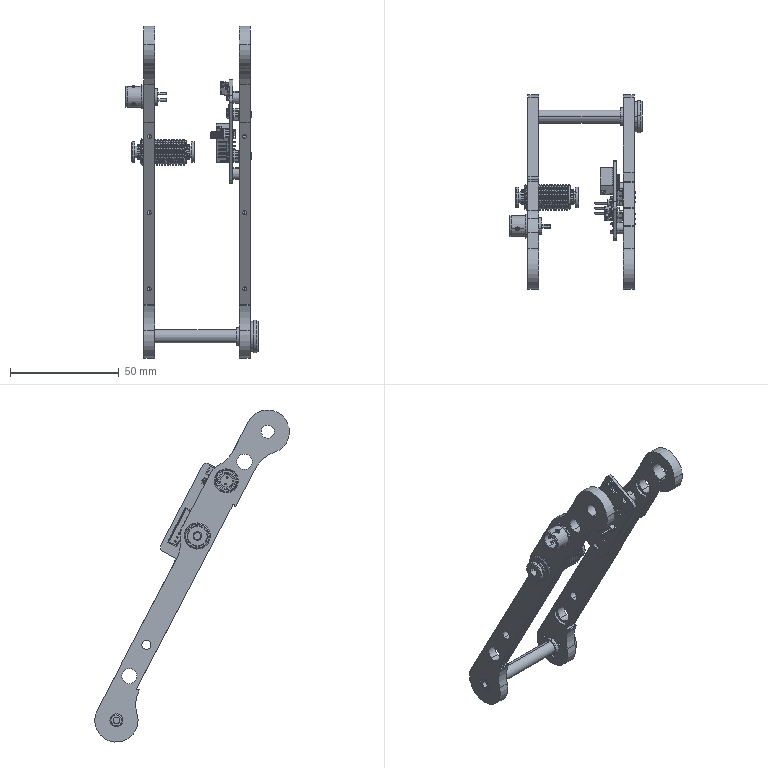Part | NX | features BREP 185 | 185 solids | 2496 faces | box 60.8 x 89.643 x 152.852 mm | volume 26403 mm3 | plane 1478 | cylinder 507 | spline 453 | sphere 28 | cone 26 | torus 4 | commonest cylinder face diameters 0.1 x102 0.06 x54 12 x33 2 x22 0.011 x18 0.39 x18